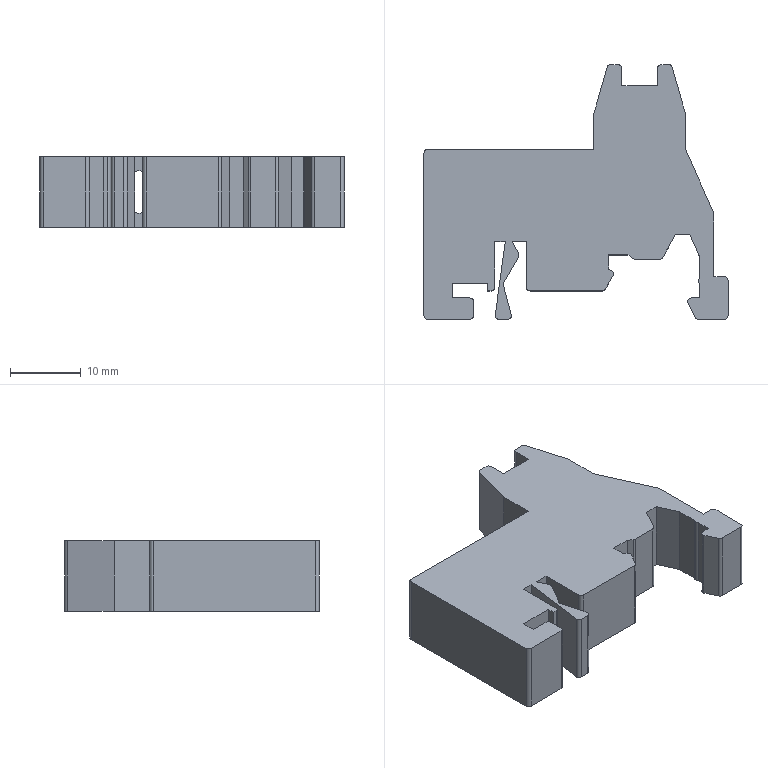Part | STEP file | terminal stopper UK2.5B | 1 solid | 83 faces | box 43 x 36 x 10 mm | volume 8109 mm3 | plane 53 | cylinder 30 | commonest cylinder face diameters 1 x26 6 x4